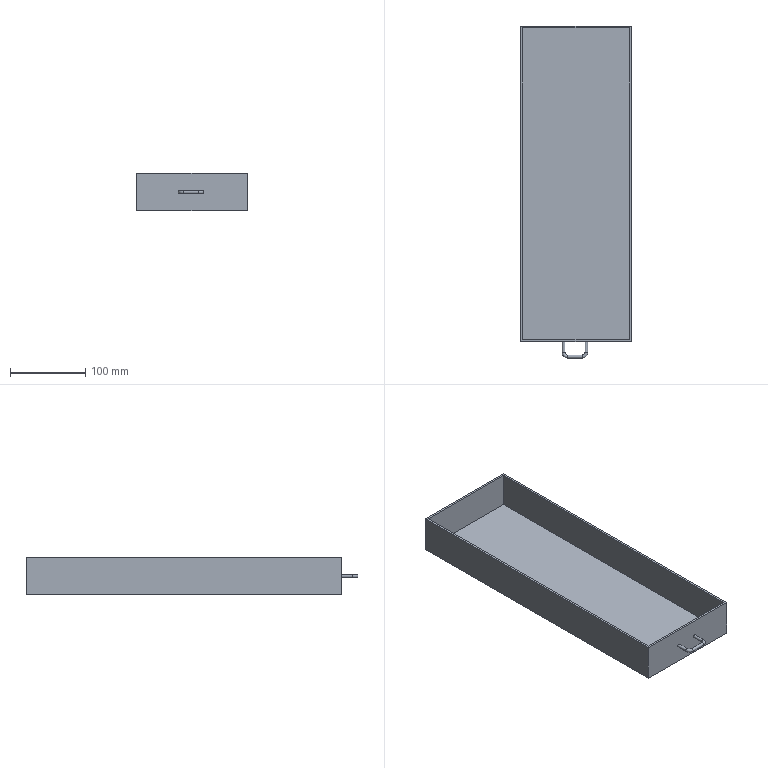Part | NX | features solid 2 | 1 solid | 16 faces | box 147 x 442 x 50 mm | volume 288651 mm3 | plane 11 | cylinder 3 | torus 2 | commonest cylinder face diameters 4 x3
STEP:
#1=CARTESIAN_POINT('',(122.,-375.,-383.));
#2=VERTEX_POINT('',#1);
#3=CARTESIAN_POINT('',(122.,-375.,-385.));
#4=DIRECTION('',(0.,1.,0.));
#5=DIRECTION('',(0.,0.,1.));
#6=AXIS2_PLACEMENT_3D('',#3,#4,#5);
#7=CIRCLE('',#6,2.);
#8=EDGE_CURVE('',#2,#2,#7,.T.);
#9=ORIENTED_EDGE('',*,*,#8,.T.);
#10=EDGE_LOOP('',(#9));
#11=FACE_BOUND('',#10,.T.);
#12=CARTESIAN_POINT('',(65.,-375.,-410.));
#13=VERTEX_POINT('',#12);
#14=CARTESIAN_POINT('',(212.,-375.,-410.));
#15=VERTEX_POINT('',#14);
#16=CARTESIAN_POINT('',(52.,-375.,-410.));
#17=DIRECTION('',(1.,0.,0.));
#18=VECTOR('',#17,1000.);
#19=LINE('',#16,#18);
#20=EDGE_CURVE('',#13,#15,#19,.T.);
#21=ORIENTED_EDGE('',*,*,#20,.T.);
#22=CARTESIAN_POINT('',(212.,-375.,-360.));
#23=VERTEX_POINT('',#22);
#24=CARTESIAN_POINT('',(212.,-375.,-360.));
#25=DIRECTION('',(0.,0.,-1.));
#26=VECTOR('',#25,1000.);
#27=LINE('',#24,#26);
#28=EDGE_CURVE('',#23,#15,#27,.T.);
#29=ORIENTED_EDGE('',*,*,#28,.F.);
#30=CARTESIAN_POINT('',(65.,-375.,-360.));
#31=VERTEX_POINT('',#30);
#32=CARTESIAN_POINT('',(52.,-375.,-360.));
#33=DIRECTION('',(1.,0.,0.));
#34=VECTOR('',#33,1000.);
#35=LINE('',#32,#34);
#36=EDGE_CURVE('',#31,#23,#35,.T.);
#37=ORIENTED_EDGE('',*,*,#36,.F.);
#38=CARTESIAN_POINT('',(65.,-375.,-300.));
#39=DIRECTION('',(0.,0.,-1.));
#40=VECTOR('',#39,1000.);
#41=LINE('',#38,#40);
#42=EDGE_CURVE('',#31,#13,#41,.T.);
#43=ORIENTED_EDGE('',*,*,#42,.T.);
#44=EDGE_LOOP('',(#21,#29,#37,#43));
#45=FACE_BOUND('',#44,.T.);
#46=CARTESIAN_POINT('',(152.,-375.,-383.));
#47=VERTEX_POINT('',#46);
#48=CARTESIAN_POINT('',(152.,-375.,-385.));
#49=DIRECTION('',(0.,1.,0.));
#50=DIRECTION('',(0.,0.,1.));
#51=AXIS2_PLACEMENT_3D('',#48,#49,#50);
#52=CIRCLE('',#51,2.);
#53=EDGE_CURVE('',#47,#47,#52,.T.);
#54=ORIENTED_EDGE('',*,*,#53,.T.);
#55=EDGE_LOOP('',(#54));
#56=FACE_BOUND('',#55,.T.);
#57=CARTESIAN_POINT('',(52.,-375.,-360.));
#58=DIRECTION('',(0.,-1.,0.));
#59=DIRECTION('',(0.,0.,1.));
#60=AXIS2_PLACEMENT_3D('',#57,#58,#59);
#61=PLANE('',#60);
#62=ADVANCED_FACE('',(#11,#45,#56),#61,.T.);
#63=CARTESIAN_POINT('',(209.5,-372.5,-407.5));
#64=VERTEX_POINT('',#63);
#65=CARTESIAN_POINT('',(209.5,42.5,-407.5));
#66=VERTEX_POINT('',#65);
#67=CARTESIAN_POINT('',(209.5,-252.5,-407.5));
#68=DIRECTION('',(0.,1.,0.));
#69=VECTOR('',#68,1000.);
#70=LINE('',#67,#69);
#71=EDGE_CURVE('',#64,#66,#70,.T.);
#72=ORIENTED_EDGE('',*,*,#71,.T.);
#73=CARTESIAN_POINT('',(67.5,42.5,-407.5));
#74=VERTEX_POINT('',#73);
#75=CARTESIAN_POINT('',(199.5,42.5,-407.5));
#76=DIRECTION('',(-1.,0.,0.));
#77=VECTOR('',#76,1000.);
#78=LINE('',#75,#77);
#79=EDGE_CURVE('',#66,#74,#78,.T.);
#80=ORIENTED_EDGE('',*,*,#79,.T.);
#81=CARTESIAN_POINT('',(67.5,-372.5,-407.5));
#82=VERTEX_POINT('',#81);
#83=CARTESIAN_POINT('',(67.5,-252.5,-407.5));
#84=DIRECTION('',(0.,-1.,0.));
#85=VECTOR('',#84,1000.);
#86=LINE('',#83,#85);
#87=EDGE_CURVE('',#74,#82,#86,.T.);
#88=ORIENTED_EDGE('',*,*,#87,.T.);
#89=CARTESIAN_POINT('',(199.5,-372.5,-407.5));
#90=DIRECTION('',(1.,0.,0.));
#91=VECTOR('',#90,1000.);
#92=LINE('',#89,#91);
#93=EDGE_CURVE('',#82,#64,#92,.T.);
#94=ORIENTED_EDGE('',*,*,#93,.T.);
#95=EDGE_LOOP('',(#72,#80,#88,#94));
#96=FACE_BOUND('',#95,.T.);
#97=CARTESIAN_POINT('',(199.5,-252.5,-407.5));
#98=DIRECTION('',(0.,0.,-1.));
#99=DIRECTION('',(-1.,0.,0.));
#100=AXIS2_PLACEMENT_3D('',#97,#98,#99);
#101=PLANE('',#100);
#102=ADVANCED_FACE('',(#96),#101,.F.);
#103=CARTESIAN_POINT('',(212.,45.,-410.));
#104=VERTEX_POINT('',#103);
#105=CARTESIAN_POINT('',(65.,45.,-410.));
#106=VERTEX_POINT('',#105);
#107=CARTESIAN_POINT('',(202.,45.,-410.));
#108=DIRECTION('',(-1.,0.,0.));
#109=VECTOR('',#108,1000.);
#110=LINE('',#107,#109);
#111=EDGE_CURVE('',#104,#106,#110,.T.);
#112=ORIENTED_EDGE('',*,*,#111,.F.);
#113=CARTESIAN_POINT('',(212.,-182.5,-410.));
#114=DIRECTION('',(0.,1.,0.));
#115=VECTOR('',#114,1000.);
#116=LINE('',#113,#115);
#117=EDGE_CURVE('',#15,#104,#116,.T.);
#118=ORIENTED_EDGE('',*,*,#117,.F.);
#119=ORIENTED_EDGE('',*,*,#20,.F.);
#120=CARTESIAN_POINT('',(65.,-182.5,-410.));
#121=DIRECTION('',(0.,-1.,0.));
#122=VECTOR('',#121,1000.);
#123=LINE('',#120,#122);
#124=EDGE_CURVE('',#106,#13,#123,.T.);
#125=ORIENTED_EDGE('',*,*,#124,.F.);
#126=EDGE_LOOP('',(#112,#118,#119,#125));
#127=FACE_BOUND('',#126,.T.);
#128=CARTESIAN_POINT('',(199.5,-182.5,-410.));
#129=DIRECTION('',(0.,0.,-1.));
#130=DIRECTION('',(-1.,0.,0.));
#131=AXIS2_PLACEMENT_3D('',#128,#129,#130);
#132=PLANE('',#131);
#133=ADVANCED_FACE('',(#127),#132,.T.);
#134=CARTESIAN_POINT('',(209.5,-372.5,-360.));
#135=VERTEX_POINT('',#134);
#136=CARTESIAN_POINT('',(209.5,-372.5,-360.));
#137=DIRECTION('',(0.,0.,-1.));
#138=VECTOR('',#137,1000.);
#139=LINE('',#136,#138);
#140=EDGE_CURVE('',#135,#64,#139,.T.);
#141=ORIENTED_EDGE('',*,*,#140,.T.);
#142=ORIENTED_EDGE('',*,*,#93,.F.);
#143=CARTESIAN_POINT('',(67.5,-372.5,-360.));
#144=VERTEX_POINT('',#143);
#145=CARTESIAN_POINT('',(67.5,-372.5,-360.));
#146=DIRECTION('',(0.,0.,-1.));
#147=VECTOR('',#146,1000.);
#148=LINE('',#145,#147);
#149=EDGE_CURVE('',#144,#82,#148,.T.);
#150=ORIENTED_EDGE('',*,*,#149,.F.);
#151=CARTESIAN_POINT('',(202.,-372.5,-360.));
#152=DIRECTION('',(-1.,0.,0.));
#153=VECTOR('',#152,1000.);
#154=LINE('',#151,#153);
#155=EDGE_CURVE('',#135,#144,#154,.T.);
#156=ORIENTED_EDGE('',*,*,#155,.F.);
#157=EDGE_LOOP('',(#141,#142,#150,#156));
#158=FACE_BOUND('',#157,.T.);
#159=CARTESIAN_POINT('',(202.,-372.5,-360.));
#160=DIRECTION('',(0.,1.,0.));
#161=DIRECTION('',(0.,0.,-1.));
#162=AXIS2_PLACEMENT_3D('',#159,#160,#161);
#163=PLANE('',#162);
#164=ADVANCED_FACE('',(#158),#163,.T.);
#165=ORIENTED_EDGE('',*,*,#117,.T.);
#166=CARTESIAN_POINT('',(212.,45.,-360.));
#167=VERTEX_POINT('',#166);
#168=CARTESIAN_POINT('',(212.,45.,-360.));
#169=DIRECTION('',(0.,0.,-1.));
#170=VECTOR('',#169,1000.);
#171=LINE('',#168,#170);
#172=EDGE_CURVE('',#167,#104,#171,.T.);
#173=ORIENTED_EDGE('',*,*,#172,.F.);
#174=CARTESIAN_POINT('',(212.,-372.5,-360.));
#175=DIRECTION('',(0.,1.,0.));
#176=VECTOR('',#175,1000.);
#177=LINE('',#174,#176);
#178=EDGE_CURVE('',#23,#167,#177,.T.);
#179=ORIENTED_EDGE('',*,*,#178,.F.);
#180=ORIENTED_EDGE('',*,*,#28,.T.);
#181=EDGE_LOOP('',(#165,#173,#179,#180));
#182=FACE_BOUND('',#181,.T.);
#183=CARTESIAN_POINT('',(212.,-375.,-360.));
#184=DIRECTION('',(1.,0.,0.));
#185=DIRECTION('',(0.,0.,-1.));
#186=AXIS2_PLACEMENT_3D('',#183,#184,#185);
#187=PLANE('',#186);
#188=ADVANCED_FACE('',(#182),#187,.T.);
#189=ORIENTED_EDGE('',*,*,#124,.T.);
#190=ORIENTED_EDGE('',*,*,#42,.F.);
#191=CARTESIAN_POINT('',(65.,45.,-360.));
#192=VERTEX_POINT('',#191);
#193=CARTESIAN_POINT('',(65.,-372.5,-360.));
#194=DIRECTION('',(0.,-1.,0.));
#195=VECTOR('',#194,1000.);
#196=LINE('',#193,#195);
#197=EDGE_CURVE('',#192,#31,#196,.T.);
#198=ORIENTED_EDGE('',*,*,#197,.F.);
#199=CARTESIAN_POINT('',(65.,45.,-360.));
#200=DIRECTION('',(0.,0.,-1.));
#201=VECTOR('',#200,1000.);
#202=LINE('',#199,#201);
#203=EDGE_CURVE('',#192,#106,#202,.T.);
#204=ORIENTED_EDGE('',*,*,#203,.T.);
#205=EDGE_LOOP('',(#189,#190,#198,#204));
#206=FACE_BOUND('',#205,.T.);
#207=CARTESIAN_POINT('',(65.,80.624,-300.));
#208=DIRECTION('',(1.,0.,0.));
#209=DIRECTION('',(0.,0.,-1.));
#210=AXIS2_PLACEMENT_3D('',#207,#208,#209);
#211=PLANE('',#210);
#212=ADVANCED_FACE('',(#206),#211,.F.);
#213=ORIENTED_EDGE('',*,*,#155,.T.);
#214=CARTESIAN_POINT('',(67.5,42.5,-360.));
#215=VERTEX_POINT('',#214);
#216=CARTESIAN_POINT('',(67.5,80.624,-360.));
#217=DIRECTION('',(0.,1.,0.));
#218=VECTOR('',#217,1000.);
#219=LINE('',#216,#218);
#220=EDGE_CURVE('',#144,#215,#219,.T.);
#221=ORIENTED_EDGE('',*,*,#220,.T.);
#222=CARTESIAN_POINT('',(209.5,42.5,-360.));
#223=VERTEX_POINT('',#222);
#224=CARTESIAN_POINT('',(52.,42.5,-360.));
#225=DIRECTION('',(1.,0.,0.));
#226=VECTOR('',#225,1000.);
#227=LINE('',#224,#226);
#228=EDGE_CURVE('',#215,#223,#227,.T.);
#229=ORIENTED_EDGE('',*,*,#228,.T.);
#230=CARTESIAN_POINT('',(209.5,-372.5,-360.));
#231=DIRECTION('',(0.,-1.,0.));
#232=VECTOR('',#231,1000.);
#233=LINE('',#230,#232);
#234=EDGE_CURVE('',#223,#135,#233,.T.);
#235=ORIENTED_EDGE('',*,*,#234,.T.);
#236=EDGE_LOOP('',(#213,#221,#229,#235));
#237=FACE_BOUND('',#236,.T.);
#238=ORIENTED_EDGE('',*,*,#178,.T.);
#239=CARTESIAN_POINT('',(202.,45.,-360.));
#240=DIRECTION('',(-1.,0.,0.));
#241=VECTOR('',#240,1000.);
#242=LINE('',#239,#241);
#243=EDGE_CURVE('',#167,#192,#242,.T.);
#244=ORIENTED_EDGE('',*,*,#243,.T.);
#245=ORIENTED_EDGE('',*,*,#197,.T.);
#246=ORIENTED_EDGE('',*,*,#36,.T.);
#247=EDGE_LOOP('',(#238,#244,#245,#246));
#248=FACE_BOUND('',#247,.T.);
#249=CARTESIAN_POINT('',(202.,-372.5,-360.));
#250=DIRECTION('',(0.,0.,-1.));
#251=DIRECTION('',(-1.,0.,0.));
#252=AXIS2_PLACEMENT_3D('',#249,#250,#251);
#253=PLANE('',#252);
#254=ADVANCED_FACE('',(#237,#248),#253,.F.);
#255=CARTESIAN_POINT('',(209.5,42.5,-360.));
#256=DIRECTION('',(0.,0.,-1.));
#257=VECTOR('',#256,1000.);
#258=LINE('',#255,#257);
#259=EDGE_CURVE('',#223,#66,#258,.T.);
#260=ORIENTED_EDGE('',*,*,#259,.F.);
#261=ORIENTED_EDGE('',*,*,#228,.F.);
#262=CARTESIAN_POINT('',(67.5,42.5,-300.));
#263=DIRECTION('',(0.,0.,-1.));
#264=VECTOR('',#263,1000.);
#265=LINE('',#262,#264);
#266=EDGE_CURVE('',#215,#74,#265,.T.);
#267=ORIENTED_EDGE('',*,*,#266,.T.);
#268=ORIENTED_EDGE('',*,*,#79,.F.);
#269=EDGE_LOOP('',(#260,#261,#267,#268));
#270=FACE_BOUND('',#269,.T.);
#271=CARTESIAN_POINT('',(52.,42.5,-360.));
#272=DIRECTION('',(0.,-1.,0.));
#273=DIRECTION('',(0.,0.,1.));
#274=AXIS2_PLACEMENT_3D('',#271,#272,#273);
#275=PLANE('',#274);
#276=ADVANCED_FACE('',(#270),#275,.T.);
#277=ORIENTED_EDGE('',*,*,#111,.T.);
#278=ORIENTED_EDGE('',*,*,#203,.F.);
#279=ORIENTED_EDGE('',*,*,#243,.F.);
#280=ORIENTED_EDGE('',*,*,#172,.T.);
#281=EDGE_LOOP('',(#277,#278,#279,#280));
#282=FACE_BOUND('',#281,.T.);
#283=CARTESIAN_POINT('',(202.,45.,-360.));
#284=DIRECTION('',(0.,1.,0.));
#285=DIRECTION('',(0.,0.,-1.));
#286=AXIS2_PLACEMENT_3D('',#283,#284,#285);
#287=PLANE('',#286);
#288=ADVANCED_FACE('',(#282),#287,.T.);
#289=ORIENTED_EDGE('',*,*,#87,.F.);
#290=ORIENTED_EDGE('',*,*,#266,.F.);
#291=ORIENTED_EDGE('',*,*,#220,.F.);
#292=ORIENTED_EDGE('',*,*,#149,.T.);
#293=EDGE_LOOP('',(#289,#290,#291,#292));
#294=FACE_BOUND('',#293,.T.);
#295=CARTESIAN_POINT('',(67.5,10.624,-300.));
#296=DIRECTION('',(1.,0.,0.));
#297=DIRECTION('',(0.,0.,-1.));
#298=AXIS2_PLACEMENT_3D('',#295,#296,#297);
#299=PLANE('',#298);
#300=ADVANCED_FACE('',(#294),#299,.T.);
#301=ORIENTED_EDGE('',*,*,#71,.F.);
#302=ORIENTED_EDGE('',*,*,#140,.F.);
#303=ORIENTED_EDGE('',*,*,#234,.F.);
#304=ORIENTED_EDGE('',*,*,#259,.T.);
#305=EDGE_LOOP('',(#301,#302,#303,#304));
#306=FACE_BOUND('',#305,.T.);
#307=CARTESIAN_POINT('',(209.5,-252.5,-360.));
#308=DIRECTION('',(-1.,0.,0.));
#309=DIRECTION('',(0.,0.,1.));
#310=AXIS2_PLACEMENT_3D('',#307,#308,#309);
#311=PLANE('',#310);
#312=ADVANCED_FACE('',(#306),#311,.T.);
#313=CARTESIAN_POINT('',(122.,-390.,-383.));
#314=VERTEX_POINT('',#313);
#315=CARTESIAN_POINT('',(122.,-390.,-385.));
#316=DIRECTION('',(0.,-1.,0.));
#317=DIRECTION('',(0.,0.,1.));
#318=AXIS2_PLACEMENT_3D('',#315,#316,#317);
#319=CIRCLE('',#318,2.);
#320=EDGE_CURVE('',#314,#314,#319,.T.);
#321=ORIENTED_EDGE('',*,*,#320,.F.);
#322=EDGE_LOOP('',(#321));
#323=FACE_BOUND('',#322,.T.);
#324=ORIENTED_EDGE('',*,*,#8,.F.);
#325=EDGE_LOOP('',(#324));
#326=FACE_BOUND('',#325,.T.);
#327=CARTESIAN_POINT('',(122.,-390.,-385.));
#328=DIRECTION('',(0.,1.,0.));
#329=DIRECTION('',(0.,0.,-1.));
#330=AXIS2_PLACEMENT_3D('',#327,#328,#329);
#331=CYLINDRICAL_SURFACE('',#330,2.);
#332=ADVANCED_FACE('',(#323,#326),#331,.T.);
#333=CARTESIAN_POINT('',(127.,-395.,-383.));
#334=VERTEX_POINT('',#333);
#335=CARTESIAN_POINT('',(127.,-395.,-385.));
#336=DIRECTION('',(1.,0.,0.));
#337=DIRECTION('',(0.,0.,1.));
#338=AXIS2_PLACEMENT_3D('',#335,#336,#337);
#339=CIRCLE('',#338,2.);
#340=EDGE_CURVE('',#334,#334,#339,.T.);
#341=ORIENTED_EDGE('',*,*,#340,.F.);
#342=EDGE_LOOP('',(#341));
#343=FACE_BOUND('',#342,.T.);
#344=ORIENTED_EDGE('',*,*,#320,.T.);
#345=EDGE_LOOP('',(#344));
#346=FACE_BOUND('',#345,.T.);
#347=CARTESIAN_POINT('',(127.,-390.,-385.));
#348=DIRECTION('',(0.,0.,1.));
#349=DIRECTION('',(1.,0.,0.));
#350=AXIS2_PLACEMENT_3D('',#347,#348,#349);
#351=TOROIDAL_SURFACE('',#350,5.,2.);
#352=ADVANCED_FACE('',(#343,#346),#351,.T.);
#353=CARTESIAN_POINT('',(147.,-395.,-383.));
#354=VERTEX_POINT('',#353);
#355=CARTESIAN_POINT('',(147.,-395.,-385.));
#356=DIRECTION('',(1.,0.,0.));
#357=DIRECTION('',(0.,0.,1.));
#358=AXIS2_PLACEMENT_3D('',#355,#356,#357);
#359=CIRCLE('',#358,2.);
#360=EDGE_CURVE('',#354,#354,#359,.T.);
#361=ORIENTED_EDGE('',*,*,#360,.F.);
#362=EDGE_LOOP('',(#361));
#363=FACE_BOUND('',#362,.T.);
#364=ORIENTED_EDGE('',*,*,#340,.T.);
#365=EDGE_LOOP('',(#364));
#366=FACE_BOUND('',#365,.T.);
#367=CARTESIAN_POINT('',(147.,-395.,-385.));
#368=DIRECTION('',(-1.,0.,0.));
#369=DIRECTION('',(0.,0.,1.));
#370=AXIS2_PLACEMENT_3D('',#367,#368,#369);
#371=CYLINDRICAL_SURFACE('',#370,2.);
#372=ADVANCED_FACE('',(#363,#366),#371,.T.);
#373=CARTESIAN_POINT('',(152.,-390.,-383.));
#374=VERTEX_POINT('',#373);
#375=CARTESIAN_POINT('',(152.,-390.,-385.));
#376=DIRECTION('',(0.,1.,0.));
#377=DIRECTION('',(0.,0.,1.));
#378=AXIS2_PLACEMENT_3D('',#375,#376,#377);
#379=CIRCLE('',#378,2.);
#380=EDGE_CURVE('',#374,#374,#379,.T.);
#381=ORIENTED_EDGE('',*,*,#380,.F.);
#382=EDGE_LOOP('',(#381));
#383=FACE_BOUND('',#382,.T.);
#384=ORIENTED_EDGE('',*,*,#360,.T.);
#385=EDGE_LOOP('',(#384));
#386=FACE_BOUND('',#385,.T.);
#387=CARTESIAN_POINT('',(147.,-390.,-385.));
#388=DIRECTION('',(0.,0.,1.));
#389=DIRECTION('',(1.,0.,0.));
#390=AXIS2_PLACEMENT_3D('',#387,#388,#389);
#391=TOROIDAL_SURFACE('',#390,5.,2.);
#392=ADVANCED_FACE('',(#383,#386),#391,.T.);
#393=ORIENTED_EDGE('',*,*,#380,.T.);
#394=EDGE_LOOP('',(#393));
#395=FACE_BOUND('',#394,.T.);
#396=ORIENTED_EDGE('',*,*,#53,.F.);
#397=EDGE_LOOP('',(#396));
#398=FACE_BOUND('',#397,.T.);
#399=CARTESIAN_POINT('',(152.,-390.,-385.));
#400=DIRECTION('',(0.,1.,0.));
#401=DIRECTION('',(0.,0.,-1.));
#402=AXIS2_PLACEMENT_3D('',#399,#400,#401);
#403=CYLINDRICAL_SURFACE('',#402,2.);
#404=ADVANCED_FACE('',(#395,#398),#403,.T.);
#405=CLOSED_SHELL('',(#62,#102,#133,#164,#188,#212,#254,#276,#288,#300,#312,#332,#352,#372,#392,#404));
#406=MANIFOLD_SOLID_BREP('',#405);
#407=(LENGTH_UNIT()NAMED_UNIT(*)SI_UNIT(.MILLI.,.METRE.));
#408=UNCERTAINTY_MEASURE_WITH_UNIT(LENGTH_MEASURE(0.00001),#407,'','');
#409=(NAMED_UNIT(*)PLANE_ANGLE_UNIT()SI_UNIT($,.RADIAN.));
#410=(NAMED_UNIT(*)SI_UNIT($,.STERADIAN.)SOLID_ANGLE_UNIT());
#411=(GEOMETRIC_REPRESENTATION_CONTEXT(3)GLOBAL_UNCERTAINTY_ASSIGNED_CONTEXT((#408))GLOBAL_UNIT_ASSIGNED_CONTEXT((#407,#409,#410))REPRESENTATION_CONTEXT('',''));
#412=ADVANCED_BREP_SHAPE_REPRESENTATION('',(#406),#411);